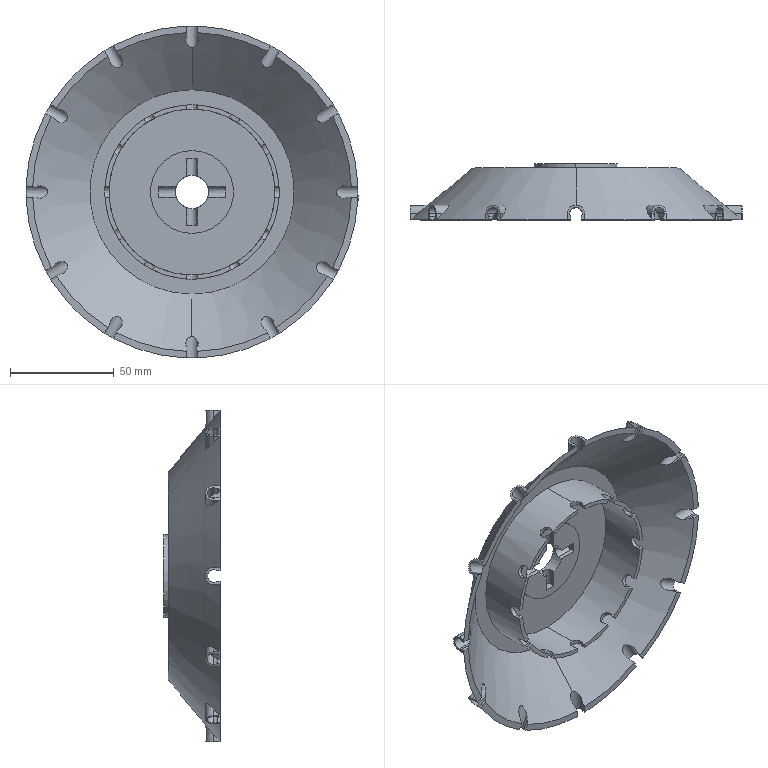Part | SolidWorks | features ICE 6, CirPattern 3, Revolution 1, Shell 1 | 1 solid | 227 faces | box 160 x 27 x 160 mm | volume 59816 mm3 | plane 125 | cylinder 98 | cone 4 | commonest cylinder face diameters 6 x72 8 x12 5 x4 40 x4 16 x2 80 x2